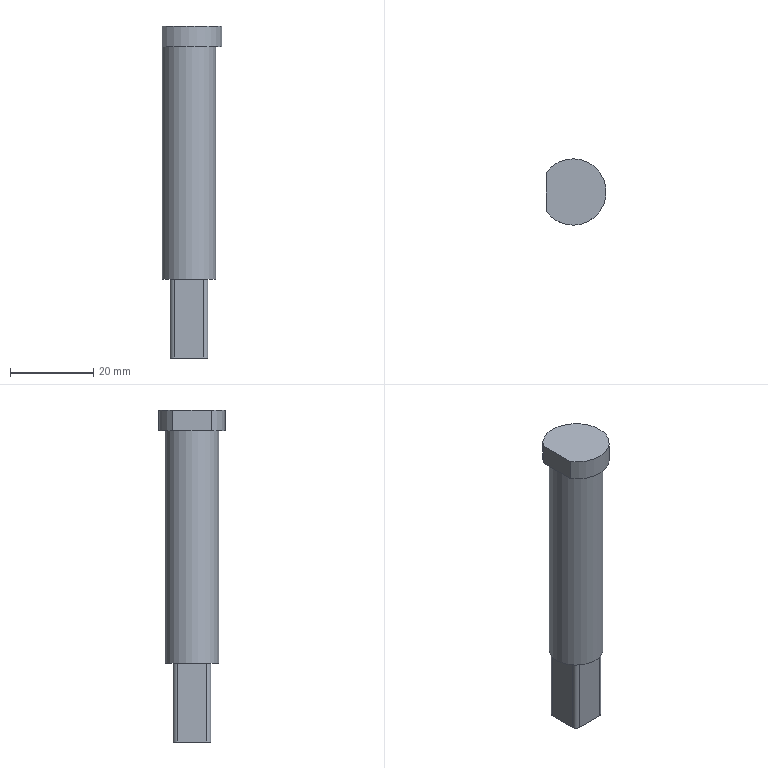Part | NX | features solid 2 | 1 solid | 15 faces | box 14.5 x 16 x 80 mm | volume 9946 mm3 | plane 9 | cylinder 6 | commonest cylinder face diameters 2.1 x4 13 x1 16 x1
STEP:
#1=CARTESIAN_POINT('',(-674.255,-597.733,33.));
#2=VERTEX_POINT('',#1);
#3=CARTESIAN_POINT('',(-680.755,-597.733,33.));
#4=DIRECTION('',(0.,0.,1.));
#5=DIRECTION('',(1.,0.,0.));
#6=AXIS2_PLACEMENT_3D('',#3,#4,#5);
#7=CIRCLE('',#6,6.5);
#8=EDGE_CURVE('',#2,#2,#7,.T.);
#9=ORIENTED_EDGE('',*,*,#8,.T.);
#10=EDGE_LOOP('',(#9));
#11=FACE_BOUND('',#10,.T.);
#12=CARTESIAN_POINT('',(-687.255,-597.733,89.));
#13=VERTEX_POINT('',#12);
#14=CARTESIAN_POINT('',(-680.755,-597.733,89.));
#15=DIRECTION('',(0.,0.,1.));
#16=DIRECTION('',(1.,0.,0.));
#17=AXIS2_PLACEMENT_3D('',#14,#15,#16);
#18=CIRCLE('',#17,6.5);
#19=EDGE_CURVE('',#13,#13,#18,.T.);
#20=ORIENTED_EDGE('',*,*,#19,.F.);
#21=EDGE_LOOP('',(#20));
#22=FACE_BOUND('',#21,.T.);
#23=CARTESIAN_POINT('',(-680.755,-597.733,94.));
#24=DIRECTION('',(0.,0.,-1.));
#25=DIRECTION('',(-1.,0.,0.));
#26=AXIS2_PLACEMENT_3D('',#23,#24,#25);
#27=CYLINDRICAL_SURFACE('',#26,6.5);
#28=ADVANCED_FACE('',(#11,#22),#27,.T.);
#29=CARTESIAN_POINT('',(-677.255,-593.183,33.));
#30=VERTEX_POINT('',#29);
#31=CARTESIAN_POINT('',(-684.255,-593.183,33.));
#32=VERTEX_POINT('',#31);
#33=CARTESIAN_POINT('',(-676.205,-593.183,33.));
#34=DIRECTION('',(-1.,0.,0.));
#35=VECTOR('',#34,1000.);
#36=LINE('',#33,#35);
#37=EDGE_CURVE('',#30,#32,#36,.T.);
#38=ORIENTED_EDGE('',*,*,#37,.T.);
#39=CARTESIAN_POINT('',(-685.305,-594.233,33.));
#40=VERTEX_POINT('',#39);
#41=CARTESIAN_POINT('',(-684.255,-594.233,33.));
#42=DIRECTION('',(0.,0.,1.));
#43=DIRECTION('',(1.,0.,0.));
#44=AXIS2_PLACEMENT_3D('',#41,#42,#43);
#45=CIRCLE('',#44,1.05);
#46=EDGE_CURVE('',#32,#40,#45,.T.);
#47=ORIENTED_EDGE('',*,*,#46,.T.);
#48=CARTESIAN_POINT('',(-685.305,-601.233,33.));
#49=VERTEX_POINT('',#48);
#50=CARTESIAN_POINT('',(-685.305,-593.183,33.));
#51=DIRECTION('',(0.,-1.,0.));
#52=VECTOR('',#51,1000.);
#53=LINE('',#50,#52);
#54=EDGE_CURVE('',#40,#49,#53,.T.);
#55=ORIENTED_EDGE('',*,*,#54,.T.);
#56=CARTESIAN_POINT('',(-684.255,-602.283,33.));
#57=VERTEX_POINT('',#56);
#58=CARTESIAN_POINT('',(-684.255,-601.233,33.));
#59=DIRECTION('',(0.,0.,1.));
#60=DIRECTION('',(1.,0.,0.));
#61=AXIS2_PLACEMENT_3D('',#58,#59,#60);
#62=CIRCLE('',#61,1.05);
#63=EDGE_CURVE('',#49,#57,#62,.T.);
#64=ORIENTED_EDGE('',*,*,#63,.T.);
#65=CARTESIAN_POINT('',(-677.255,-602.283,33.));
#66=VERTEX_POINT('',#65);
#67=CARTESIAN_POINT('',(-685.305,-602.283,33.));
#68=DIRECTION('',(1.,0.,0.));
#69=VECTOR('',#68,1000.);
#70=LINE('',#67,#69);
#71=EDGE_CURVE('',#57,#66,#70,.T.);
#72=ORIENTED_EDGE('',*,*,#71,.T.);
#73=CARTESIAN_POINT('',(-676.205,-601.233,33.));
#74=VERTEX_POINT('',#73);
#75=CARTESIAN_POINT('',(-677.255,-601.233,33.));
#76=DIRECTION('',(0.,0.,1.));
#77=DIRECTION('',(1.,0.,0.));
#78=AXIS2_PLACEMENT_3D('',#75,#76,#77);
#79=CIRCLE('',#78,1.05);
#80=EDGE_CURVE('',#66,#74,#79,.T.);
#81=ORIENTED_EDGE('',*,*,#80,.T.);
#82=CARTESIAN_POINT('',(-676.205,-594.233,33.));
#83=VERTEX_POINT('',#82);
#84=CARTESIAN_POINT('',(-676.205,-593.183,33.));
#85=DIRECTION('',(0.,-1.,0.));
#86=VECTOR('',#85,1000.);
#87=LINE('',#84,#86);
#88=EDGE_CURVE('',#83,#74,#87,.T.);
#89=ORIENTED_EDGE('',*,*,#88,.F.);
#90=CARTESIAN_POINT('',(-677.255,-594.233,33.));
#91=DIRECTION('',(0.,0.,1.));
#92=DIRECTION('',(1.,0.,0.));
#93=AXIS2_PLACEMENT_3D('',#90,#91,#92);
#94=CIRCLE('',#93,1.05);
#95=EDGE_CURVE('',#83,#30,#94,.T.);
#96=ORIENTED_EDGE('',*,*,#95,.T.);
#97=EDGE_LOOP('',(#38,#47,#55,#64,#72,#81,#89,#96));
#98=FACE_BOUND('',#97,.T.);
#99=ORIENTED_EDGE('',*,*,#8,.F.);
#100=EDGE_LOOP('',(#99));
#101=FACE_BOUND('',#100,.T.);
#102=CARTESIAN_POINT('',(-680.755,-597.733,33.));
#103=DIRECTION('',(0.,0.,1.));
#104=DIRECTION('',(1.,0.,0.));
#105=AXIS2_PLACEMENT_3D('',#102,#103,#104);
#106=PLANE('',#105);
#107=ADVANCED_FACE('',(#98,#101),#106,.F.);
#108=CARTESIAN_POINT('',(-687.255,-602.397,89.));
#109=VERTEX_POINT('',#108);
#110=CARTESIAN_POINT('',(-687.255,-593.069,89.));
#111=VERTEX_POINT('',#110);
#112=CARTESIAN_POINT('',(-680.755,-597.733,89.));
#113=DIRECTION('',(0.,0.,1.));
#114=DIRECTION('',(1.,0.,0.));
#115=AXIS2_PLACEMENT_3D('',#112,#113,#114);
#116=CIRCLE('',#115,8.);
#117=EDGE_CURVE('',#109,#111,#116,.T.);
#118=ORIENTED_EDGE('',*,*,#117,.F.);
#119=CARTESIAN_POINT('',(-687.255,-597.733,89.));
#120=DIRECTION('',(0.,1.,0.));
#121=VECTOR('',#120,1000.);
#122=LINE('',#119,#121);
#123=EDGE_CURVE('',#109,#13,#122,.T.);
#124=ORIENTED_EDGE('',*,*,#123,.T.);
#125=ORIENTED_EDGE('',*,*,#19,.T.);
#126=CARTESIAN_POINT('',(-687.255,-597.733,89.));
#127=DIRECTION('',(0.,1.,0.));
#128=VECTOR('',#127,1000.);
#129=LINE('',#126,#128);
#130=EDGE_CURVE('',#13,#111,#129,.T.);
#131=ORIENTED_EDGE('',*,*,#130,.T.);
#132=EDGE_LOOP('',(#118,#124,#125,#131));
#133=FACE_BOUND('',#132,.T.);
#134=CARTESIAN_POINT('',(-680.755,-597.733,89.));
#135=DIRECTION('',(0.,0.,1.));
#136=DIRECTION('',(1.,0.,0.));
#137=AXIS2_PLACEMENT_3D('',#134,#135,#136);
#138=PLANE('',#137);
#139=ADVANCED_FACE('',(#133),#138,.F.);
#140=CARTESIAN_POINT('',(-687.255,-593.069,94.));
#141=VERTEX_POINT('',#140);
#142=CARTESIAN_POINT('',(-687.255,-593.069,97.));
#143=DIRECTION('',(0.,0.,-1.));
#144=VECTOR('',#143,1000.);
#145=LINE('',#142,#144);
#146=EDGE_CURVE('',#111,#141,#145,.F.);
#147=ORIENTED_EDGE('',*,*,#146,.T.);
#148=CARTESIAN_POINT('',(-687.255,-602.397,94.));
#149=VERTEX_POINT('',#148);
#150=CARTESIAN_POINT('',(-680.755,-597.733,94.));
#151=DIRECTION('',(0.,0.,1.));
#152=DIRECTION('',(1.,0.,0.));
#153=AXIS2_PLACEMENT_3D('',#150,#151,#152);
#154=CIRCLE('',#153,8.);
#155=EDGE_CURVE('',#149,#141,#154,.T.);
#156=ORIENTED_EDGE('',*,*,#155,.F.);
#157=CARTESIAN_POINT('',(-687.255,-602.397,97.));
#158=DIRECTION('',(0.,0.,-1.));
#159=VECTOR('',#158,1000.);
#160=LINE('',#157,#159);
#161=EDGE_CURVE('',#149,#109,#160,.T.);
#162=ORIENTED_EDGE('',*,*,#161,.T.);
#163=ORIENTED_EDGE('',*,*,#117,.T.);
#164=EDGE_LOOP('',(#147,#156,#162,#163));
#165=FACE_BOUND('',#164,.T.);
#166=CARTESIAN_POINT('',(-680.755,-597.733,89.));
#167=DIRECTION('',(0.,0.,1.));
#168=DIRECTION('',(1.,0.,0.));
#169=AXIS2_PLACEMENT_3D('',#166,#167,#168);
#170=CYLINDRICAL_SURFACE('',#169,8.);
#171=ADVANCED_FACE('',(#165),#170,.T.);
#172=CARTESIAN_POINT('',(-687.255,-597.733,94.));
#173=DIRECTION('',(0.,1.,0.));
#174=VECTOR('',#173,1000.);
#175=LINE('',#172,#174);
#176=EDGE_CURVE('',#149,#141,#175,.T.);
#177=ORIENTED_EDGE('',*,*,#176,.F.);
#178=ORIENTED_EDGE('',*,*,#155,.T.);
#179=EDGE_LOOP('',(#177,#178));
#180=FACE_BOUND('',#179,.T.);
#181=CARTESIAN_POINT('',(-680.755,-597.733,94.));
#182=DIRECTION('',(0.,0.,1.));
#183=DIRECTION('',(1.,0.,0.));
#184=AXIS2_PLACEMENT_3D('',#181,#182,#183);
#185=PLANE('',#184);
#186=ADVANCED_FACE('',(#180),#185,.T.);
#187=ORIENTED_EDGE('',*,*,#161,.F.);
#188=ORIENTED_EDGE('',*,*,#176,.T.);
#189=ORIENTED_EDGE('',*,*,#146,.F.);
#190=ORIENTED_EDGE('',*,*,#130,.F.);
#191=ORIENTED_EDGE('',*,*,#123,.F.);
#192=EDGE_LOOP('',(#187,#188,#189,#190,#191));
#193=FACE_BOUND('',#192,.T.);
#194=CARTESIAN_POINT('',(-687.255,-593.069,97.));
#195=DIRECTION('',(1.,0.,0.));
#196=DIRECTION('',(0.,1.,0.));
#197=AXIS2_PLACEMENT_3D('',#194,#195,#196);
#198=PLANE('',#197);
#199=ADVANCED_FACE('',(#193),#198,.F.);
#200=CARTESIAN_POINT('',(-684.255,-602.283,14.));
#201=VERTEX_POINT('',#200);
#202=CARTESIAN_POINT('',(-677.255,-602.283,14.));
#203=VERTEX_POINT('',#202);
#204=CARTESIAN_POINT('',(-685.305,-602.283,14.));
#205=DIRECTION('',(1.,0.,0.));
#206=VECTOR('',#205,1000.);
#207=LINE('',#204,#206);
#208=EDGE_CURVE('',#201,#203,#207,.T.);
#209=ORIENTED_EDGE('',*,*,#208,.T.);
#210=CARTESIAN_POINT('',(-677.255,-602.283,33.));
#211=DIRECTION('',(0.,0.,1.));
#212=VECTOR('',#211,1000.);
#213=LINE('',#210,#212);
#214=EDGE_CURVE('',#203,#66,#213,.T.);
#215=ORIENTED_EDGE('',*,*,#214,.T.);
#216=ORIENTED_EDGE('',*,*,#71,.F.);
#217=CARTESIAN_POINT('',(-684.255,-602.283,14.));
#218=DIRECTION('',(0.,0.,1.));
#219=VECTOR('',#218,1000.);
#220=LINE('',#217,#219);
#221=EDGE_CURVE('',#57,#201,#220,.F.);
#222=ORIENTED_EDGE('',*,*,#221,.T.);
#223=EDGE_LOOP('',(#209,#215,#216,#222));
#224=FACE_BOUND('',#223,.T.);
#225=CARTESIAN_POINT('',(-685.305,-602.283,14.));
#226=DIRECTION('',(0.,-1.,0.));
#227=DIRECTION('',(0.,0.,-1.));
#228=AXIS2_PLACEMENT_3D('',#225,#226,#227);
#229=PLANE('',#228);
#230=ADVANCED_FACE('',(#224),#229,.T.);
#231=CARTESIAN_POINT('',(-676.205,-594.233,14.));
#232=VERTEX_POINT('',#231);
#233=CARTESIAN_POINT('',(-676.205,-601.233,14.));
#234=VERTEX_POINT('',#233);
#235=CARTESIAN_POINT('',(-676.205,-593.183,14.));
#236=DIRECTION('',(0.,-1.,0.));
#237=VECTOR('',#236,1000.);
#238=LINE('',#235,#237);
#239=EDGE_CURVE('',#232,#234,#238,.T.);
#240=ORIENTED_EDGE('',*,*,#239,.F.);
#241=CARTESIAN_POINT('',(-676.205,-594.233,33.));
#242=DIRECTION('',(0.,0.,1.));
#243=VECTOR('',#242,1000.);
#244=LINE('',#241,#243);
#245=EDGE_CURVE('',#232,#83,#244,.T.);
#246=ORIENTED_EDGE('',*,*,#245,.T.);
#247=ORIENTED_EDGE('',*,*,#88,.T.);
#248=CARTESIAN_POINT('',(-676.205,-601.233,14.));
#249=DIRECTION('',(0.,0.,1.));
#250=VECTOR('',#249,1000.);
#251=LINE('',#248,#250);
#252=EDGE_CURVE('',#74,#234,#251,.F.);
#253=ORIENTED_EDGE('',*,*,#252,.T.);
#254=EDGE_LOOP('',(#240,#246,#247,#253));
#255=FACE_BOUND('',#254,.T.);
#256=CARTESIAN_POINT('',(-676.205,-593.183,14.));
#257=DIRECTION('',(-1.,0.,0.));
#258=DIRECTION('',(0.,0.,1.));
#259=AXIS2_PLACEMENT_3D('',#256,#257,#258);
#260=PLANE('',#259);
#261=ADVANCED_FACE('',(#255),#260,.F.);
#262=ORIENTED_EDGE('',*,*,#37,.F.);
#263=CARTESIAN_POINT('',(-677.255,-593.183,14.));
#264=VERTEX_POINT('',#263);
#265=CARTESIAN_POINT('',(-677.255,-593.183,14.));
#266=DIRECTION('',(0.,0.,1.));
#267=VECTOR('',#266,1000.);
#268=LINE('',#265,#267);
#269=EDGE_CURVE('',#30,#264,#268,.F.);
#270=ORIENTED_EDGE('',*,*,#269,.T.);
#271=CARTESIAN_POINT('',(-684.255,-593.183,14.));
#272=VERTEX_POINT('',#271);
#273=CARTESIAN_POINT('',(-676.205,-593.183,14.));
#274=DIRECTION('',(-1.,0.,0.));
#275=VECTOR('',#274,1000.);
#276=LINE('',#273,#275);
#277=EDGE_CURVE('',#264,#272,#276,.T.);
#278=ORIENTED_EDGE('',*,*,#277,.T.);
#279=CARTESIAN_POINT('',(-684.255,-593.183,14.));
#280=DIRECTION('',(0.,0.,1.));
#281=VECTOR('',#280,1000.);
#282=LINE('',#279,#281);
#283=EDGE_CURVE('',#272,#32,#282,.T.);
#284=ORIENTED_EDGE('',*,*,#283,.T.);
#285=EDGE_LOOP('',(#262,#270,#278,#284));
#286=FACE_BOUND('',#285,.T.);
#287=CARTESIAN_POINT('',(-676.205,-593.183,14.));
#288=DIRECTION('',(0.,1.,0.));
#289=DIRECTION('',(0.,0.,1.));
#290=AXIS2_PLACEMENT_3D('',#287,#288,#289);
#291=PLANE('',#290);
#292=ADVANCED_FACE('',(#286),#291,.T.);
#293=ORIENTED_EDGE('',*,*,#54,.F.);
#294=CARTESIAN_POINT('',(-685.305,-594.233,14.));
#295=VERTEX_POINT('',#294);
#296=CARTESIAN_POINT('',(-685.305,-594.233,14.));
#297=DIRECTION('',(0.,0.,1.));
#298=VECTOR('',#297,1000.);
#299=LINE('',#296,#298);
#300=EDGE_CURVE('',#40,#295,#299,.F.);
#301=ORIENTED_EDGE('',*,*,#300,.T.);
#302=CARTESIAN_POINT('',(-685.305,-601.233,14.));
#303=VERTEX_POINT('',#302);
#304=CARTESIAN_POINT('',(-685.305,-593.183,14.));
#305=DIRECTION('',(0.,-1.,0.));
#306=VECTOR('',#305,1000.);
#307=LINE('',#304,#306);
#308=EDGE_CURVE('',#295,#303,#307,.T.);
#309=ORIENTED_EDGE('',*,*,#308,.T.);
#310=CARTESIAN_POINT('',(-685.305,-601.233,14.));
#311=DIRECTION('',(0.,0.,1.));
#312=VECTOR('',#311,1000.);
#313=LINE('',#310,#312);
#314=EDGE_CURVE('',#303,#49,#313,.T.);
#315=ORIENTED_EDGE('',*,*,#314,.T.);
#316=EDGE_LOOP('',(#293,#301,#309,#315));
#317=FACE_BOUND('',#316,.T.);
#318=CARTESIAN_POINT('',(-685.305,-593.183,14.));
#319=DIRECTION('',(-1.,0.,0.));
#320=DIRECTION('',(0.,0.,1.));
#321=AXIS2_PLACEMENT_3D('',#318,#319,#320);
#322=PLANE('',#321);
#323=ADVANCED_FACE('',(#317),#322,.T.);
#324=ORIENTED_EDGE('',*,*,#277,.F.);
#325=CARTESIAN_POINT('',(-677.255,-594.233,14.));
#326=DIRECTION('',(0.,0.,-1.));
#327=DIRECTION('',(-1.,0.,0.));
#328=AXIS2_PLACEMENT_3D('',#325,#326,#327);
#329=CIRCLE('',#328,1.05);
#330=EDGE_CURVE('',#264,#232,#329,.T.);
#331=ORIENTED_EDGE('',*,*,#330,.T.);
#332=ORIENTED_EDGE('',*,*,#239,.T.);
#333=CARTESIAN_POINT('',(-677.255,-601.233,14.));
#334=DIRECTION('',(0.,0.,-1.));
#335=DIRECTION('',(-1.,0.,0.));
#336=AXIS2_PLACEMENT_3D('',#333,#334,#335);
#337=CIRCLE('',#336,1.05);
#338=EDGE_CURVE('',#234,#203,#337,.T.);
#339=ORIENTED_EDGE('',*,*,#338,.T.);
#340=ORIENTED_EDGE('',*,*,#208,.F.);
#341=CARTESIAN_POINT('',(-684.255,-601.233,14.));
#342=DIRECTION('',(0.,0.,-1.));
#343=DIRECTION('',(-1.,0.,0.));
#344=AXIS2_PLACEMENT_3D('',#341,#342,#343);
#345=CIRCLE('',#344,1.05);
#346=EDGE_CURVE('',#201,#303,#345,.T.);
#347=ORIENTED_EDGE('',*,*,#346,.T.);
#348=ORIENTED_EDGE('',*,*,#308,.F.);
#349=CARTESIAN_POINT('',(-684.255,-594.233,14.));
#350=DIRECTION('',(0.,0.,-1.));
#351=DIRECTION('',(-1.,0.,0.));
#352=AXIS2_PLACEMENT_3D('',#349,#350,#351);
#353=CIRCLE('',#352,1.05);
#354=EDGE_CURVE('',#295,#272,#353,.T.);
#355=ORIENTED_EDGE('',*,*,#354,.T.);
#356=EDGE_LOOP('',(#324,#331,#332,#339,#340,#347,#348,#355));
#357=FACE_BOUND('',#356,.T.);
#358=CARTESIAN_POINT('',(-676.205,-602.283,14.));
#359=DIRECTION('',(0.,0.,-1.));
#360=DIRECTION('',(-1.,0.,0.));
#361=AXIS2_PLACEMENT_3D('',#358,#359,#360);
#362=PLANE('',#361);
#363=ADVANCED_FACE('',(#357),#362,.T.);
#364=ORIENTED_EDGE('',*,*,#330,.F.);
#365=ORIENTED_EDGE('',*,*,#269,.F.);
#366=ORIENTED_EDGE('',*,*,#95,.F.);
#367=ORIENTED_EDGE('',*,*,#245,.F.);
#368=EDGE_LOOP('',(#364,#365,#366,#367));
#369=FACE_BOUND('',#368,.T.);
#370=CARTESIAN_POINT('',(-677.255,-594.233,14.));
#371=DIRECTION('',(0.,0.,-1.));
#372=DIRECTION('',(-1.,0.,0.));
#373=AXIS2_PLACEMENT_3D('',#370,#371,#372);
#374=CYLINDRICAL_SURFACE('',#373,1.05);
#375=ADVANCED_FACE('',(#369),#374,.T.);
#376=ORIENTED_EDGE('',*,*,#354,.F.);
#377=ORIENTED_EDGE('',*,*,#300,.F.);
#378=ORIENTED_EDGE('',*,*,#46,.F.);
#379=ORIENTED_EDGE('',*,*,#283,.F.);
#380=EDGE_LOOP('',(#376,#377,#378,#379));
#381=FACE_BOUND('',#380,.T.);
#382=CARTESIAN_POINT('',(-684.255,-594.233,14.));
#383=DIRECTION('',(0.,0.,1.));
#384=DIRECTION('',(1.,0.,0.));
#385=AXIS2_PLACEMENT_3D('',#382,#383,#384);
#386=CYLINDRICAL_SURFACE('',#385,1.05);
#387=ADVANCED_FACE('',(#381),#386,.T.);
#388=ORIENTED_EDGE('',*,*,#338,.F.);
#389=ORIENTED_EDGE('',*,*,#252,.F.);
#390=ORIENTED_EDGE('',*,*,#80,.F.);
#391=ORIENTED_EDGE('',*,*,#214,.F.);
#392=EDGE_LOOP('',(#388,#389,#390,#391));
#393=FACE_BOUND('',#392,.T.);
#394=CARTESIAN_POINT('',(-677.255,-601.233,14.));
#395=DIRECTION('',(0.,0.,-1.));
#396=DIRECTION('',(-1.,0.,0.));
#397=AXIS2_PLACEMENT_3D('',#394,#395,#396);
#398=CYLINDRICAL_SURFACE('',#397,1.05);
#399=ADVANCED_FACE('',(#393),#398,.T.);
#400=ORIENTED_EDGE('',*,*,#346,.F.);
#401=ORIENTED_EDGE('',*,*,#221,.F.);
#402=ORIENTED_EDGE('',*,*,#63,.F.);
#403=ORIENTED_EDGE('',*,*,#314,.F.);
#404=EDGE_LOOP('',(#400,#401,#402,#403));
#405=FACE_BOUND('',#404,.T.);
#406=CARTESIAN_POINT('',(-684.255,-601.233,14.));
#407=DIRECTION('',(0.,0.,1.));
#408=DIRECTION('',(1.,0.,0.));
#409=AXIS2_PLACEMENT_3D('',#406,#407,#408);
#410=CYLINDRICAL_SURFACE('',#409,1.05);
#411=ADVANCED_FACE('',(#405),#410,.T.);
#412=CLOSED_SHELL('',(#28,#107,#139,#171,#186,#199,#230,#261,#292,#323,#363,#375,#387,#399,#411));
#413=MANIFOLD_SOLID_BREP('',#412);
#414=(LENGTH_UNIT()NAMED_UNIT(*)SI_UNIT(.MILLI.,.METRE.));
#415=UNCERTAINTY_MEASURE_WITH_UNIT(LENGTH_MEASURE(0.00001),#414,'','');
#416=(NAMED_UNIT(*)PLANE_ANGLE_UNIT()SI_UNIT($,.RADIAN.));
#417=(NAMED_UNIT(*)SI_UNIT($,.STERADIAN.)SOLID_ANGLE_UNIT());
#418=(GEOMETRIC_REPRESENTATION_CONTEXT(3)GLOBAL_UNCERTAINTY_ASSIGNED_CONTEXT((#415))GLOBAL_UNIT_ASSIGNED_CONTEXT((#414,#416,#417))REPRESENTATION_CONTEXT('',''));
#419=ADVANCED_BREP_SHAPE_REPRESENTATION('',(#413),#418);